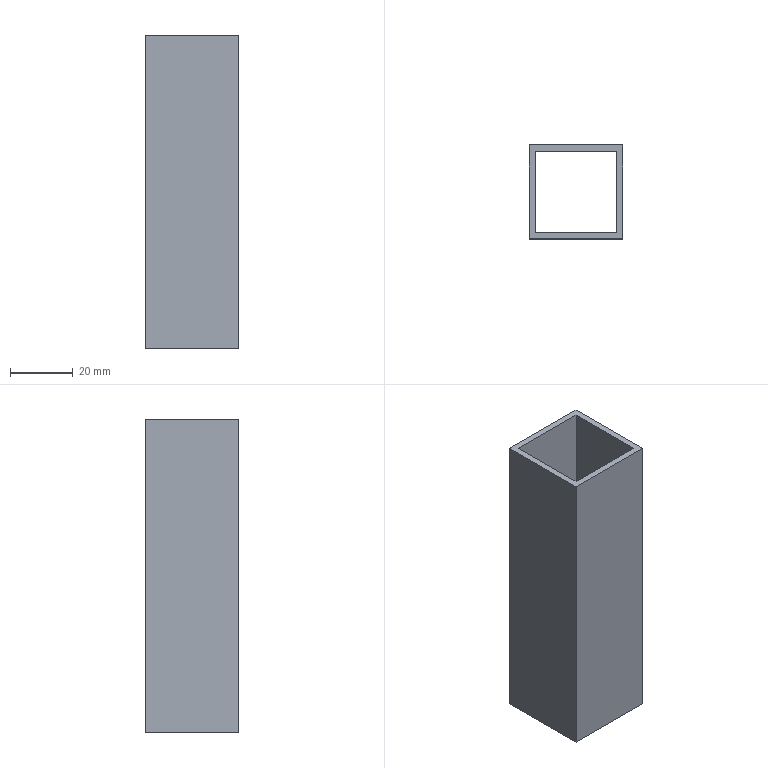Part | SolidWorks | features Extrusion 1 | 1 solid | 10 faces | box 30 x 30 x 100 mm | volume 22400 mm3 | plane 10
STEP:
#1=CARTESIAN_POINT('',(-15.,15.,50.));
#2=VERTEX_POINT('',#1);
#3=CARTESIAN_POINT('',(-15.,-15.,50.));
#4=VERTEX_POINT('',#3);
#5=CARTESIAN_POINT('',(-15.,-15.,50.));
#6=DIRECTION('',(0.,-1.,0.));
#7=VECTOR('',#6,1000.);
#8=LINE('',#5,#7);
#9=EDGE_CURVE('',#2,#4,#8,.T.);
#10=ORIENTED_EDGE('',*,*,#9,.T.);
#11=CARTESIAN_POINT('',(15.,-15.,50.));
#12=VERTEX_POINT('',#11);
#13=CARTESIAN_POINT('',(15.,-15.,50.));
#14=DIRECTION('',(1.,0.,0.));
#15=VECTOR('',#14,1000.);
#16=LINE('',#13,#15);
#17=EDGE_CURVE('',#4,#12,#16,.T.);
#18=ORIENTED_EDGE('',*,*,#17,.T.);
#19=CARTESIAN_POINT('',(15.,15.,50.));
#20=VERTEX_POINT('',#19);
#21=CARTESIAN_POINT('',(15.,-15.,50.));
#22=DIRECTION('',(0.,1.,0.));
#23=VECTOR('',#22,1000.);
#24=LINE('',#21,#23);
#25=EDGE_CURVE('',#12,#20,#24,.T.);
#26=ORIENTED_EDGE('',*,*,#25,.T.);
#27=CARTESIAN_POINT('',(15.,15.,50.));
#28=DIRECTION('',(-1.,0.,0.));
#29=VECTOR('',#28,1000.);
#30=LINE('',#27,#29);
#31=EDGE_CURVE('',#20,#2,#30,.T.);
#32=ORIENTED_EDGE('',*,*,#31,.T.);
#33=EDGE_LOOP('',(#10,#18,#26,#32));
#34=FACE_OUTER_BOUND('',#33,.T.);
#35=CARTESIAN_POINT('',(13.,-13.,50.));
#36=VERTEX_POINT('',#35);
#37=CARTESIAN_POINT('',(13.,13.,50.));
#38=VERTEX_POINT('',#37);
#39=CARTESIAN_POINT('',(13.,-13.,50.));
#40=DIRECTION('',(0.,1.,0.));
#41=VECTOR('',#40,1000.);
#42=LINE('',#39,#41);
#43=EDGE_CURVE('',#36,#38,#42,.T.);
#44=ORIENTED_EDGE('',*,*,#43,.F.);
#45=CARTESIAN_POINT('',(-13.,-13.,50.));
#46=VERTEX_POINT('',#45);
#47=CARTESIAN_POINT('',(13.,-13.,50.));
#48=DIRECTION('',(1.,0.,0.));
#49=VECTOR('',#48,1000.);
#50=LINE('',#47,#49);
#51=EDGE_CURVE('',#46,#36,#50,.T.);
#52=ORIENTED_EDGE('',*,*,#51,.F.);
#53=CARTESIAN_POINT('',(-13.,13.,50.));
#54=VERTEX_POINT('',#53);
#55=CARTESIAN_POINT('',(-13.,-13.,50.));
#56=DIRECTION('',(0.,-1.,0.));
#57=VECTOR('',#56,1000.);
#58=LINE('',#55,#57);
#59=EDGE_CURVE('',#54,#46,#58,.T.);
#60=ORIENTED_EDGE('',*,*,#59,.F.);
#61=CARTESIAN_POINT('',(13.,13.,50.));
#62=DIRECTION('',(-1.,0.,0.));
#63=VECTOR('',#62,1000.);
#64=LINE('',#61,#63);
#65=EDGE_CURVE('',#38,#54,#64,.T.);
#66=ORIENTED_EDGE('',*,*,#65,.F.);
#67=EDGE_LOOP('',(#44,#52,#60,#66));
#68=FACE_BOUND('',#67,.T.);
#69=CARTESIAN_POINT('',(0.,0.,50.));
#70=DIRECTION('',(0.,0.,1.));
#71=DIRECTION('',(1.,0.,0.));
#72=AXIS2_PLACEMENT_3D('',#69,#70,#71);
#73=PLANE('',#72);
#74=ADVANCED_FACE('',(#34,#68),#73,.T.);
#75=CARTESIAN_POINT('',(-15.,15.,-50.));
#76=VERTEX_POINT('',#75);
#77=CARTESIAN_POINT('',(-15.,-15.,-50.));
#78=VERTEX_POINT('',#77);
#79=CARTESIAN_POINT('',(-15.,-15.,-50.));
#80=DIRECTION('',(0.,-1.,0.));
#81=VECTOR('',#80,1000.);
#82=LINE('',#79,#81);
#83=EDGE_CURVE('',#76,#78,#82,.T.);
#84=ORIENTED_EDGE('',*,*,#83,.F.);
#85=CARTESIAN_POINT('',(15.,15.,-50.));
#86=VERTEX_POINT('',#85);
#87=CARTESIAN_POINT('',(15.,15.,-50.));
#88=DIRECTION('',(-1.,0.,0.));
#89=VECTOR('',#88,1000.);
#90=LINE('',#87,#89);
#91=EDGE_CURVE('',#86,#76,#90,.T.);
#92=ORIENTED_EDGE('',*,*,#91,.F.);
#93=CARTESIAN_POINT('',(15.,-15.,-50.));
#94=VERTEX_POINT('',#93);
#95=CARTESIAN_POINT('',(15.,-15.,-50.));
#96=DIRECTION('',(0.,1.,0.));
#97=VECTOR('',#96,1000.);
#98=LINE('',#95,#97);
#99=EDGE_CURVE('',#94,#86,#98,.T.);
#100=ORIENTED_EDGE('',*,*,#99,.F.);
#101=CARTESIAN_POINT('',(15.,-15.,-50.));
#102=DIRECTION('',(1.,0.,0.));
#103=VECTOR('',#102,1000.);
#104=LINE('',#101,#103);
#105=EDGE_CURVE('',#78,#94,#104,.T.);
#106=ORIENTED_EDGE('',*,*,#105,.F.);
#107=EDGE_LOOP('',(#84,#92,#100,#106));
#108=FACE_OUTER_BOUND('',#107,.T.);
#109=CARTESIAN_POINT('',(-13.,-13.,-50.));
#110=VERTEX_POINT('',#109);
#111=CARTESIAN_POINT('',(13.,-13.,-50.));
#112=VERTEX_POINT('',#111);
#113=CARTESIAN_POINT('',(13.,-13.,-50.));
#114=DIRECTION('',(1.,0.,0.));
#115=VECTOR('',#114,1000.);
#116=LINE('',#113,#115);
#117=EDGE_CURVE('',#110,#112,#116,.T.);
#118=ORIENTED_EDGE('',*,*,#117,.T.);
#119=CARTESIAN_POINT('',(13.,13.,-50.));
#120=VERTEX_POINT('',#119);
#121=CARTESIAN_POINT('',(13.,-13.,-50.));
#122=DIRECTION('',(0.,1.,0.));
#123=VECTOR('',#122,1000.);
#124=LINE('',#121,#123);
#125=EDGE_CURVE('',#112,#120,#124,.T.);
#126=ORIENTED_EDGE('',*,*,#125,.T.);
#127=CARTESIAN_POINT('',(-13.,13.,-50.));
#128=VERTEX_POINT('',#127);
#129=CARTESIAN_POINT('',(13.,13.,-50.));
#130=DIRECTION('',(-1.,0.,0.));
#131=VECTOR('',#130,1000.);
#132=LINE('',#129,#131);
#133=EDGE_CURVE('',#120,#128,#132,.T.);
#134=ORIENTED_EDGE('',*,*,#133,.T.);
#135=CARTESIAN_POINT('',(-13.,-13.,-50.));
#136=DIRECTION('',(0.,-1.,0.));
#137=VECTOR('',#136,1000.);
#138=LINE('',#135,#137);
#139=EDGE_CURVE('',#128,#110,#138,.T.);
#140=ORIENTED_EDGE('',*,*,#139,.T.);
#141=EDGE_LOOP('',(#118,#126,#134,#140));
#142=FACE_BOUND('',#141,.T.);
#143=CARTESIAN_POINT('',(0.,0.,-50.));
#144=DIRECTION('',(0.,0.,1.));
#145=DIRECTION('',(1.,0.,0.));
#146=AXIS2_PLACEMENT_3D('',#143,#144,#145);
#147=PLANE('',#146);
#148=ADVANCED_FACE('',(#108,#142),#147,.F.);
#149=ORIENTED_EDGE('',*,*,#83,.T.);
#150=CARTESIAN_POINT('',(-15.,-15.,50.));
#151=DIRECTION('',(0.,0.,-1.));
#152=VECTOR('',#151,1000.);
#153=LINE('',#150,#152);
#154=EDGE_CURVE('',#4,#78,#153,.T.);
#155=ORIENTED_EDGE('',*,*,#154,.F.);
#156=ORIENTED_EDGE('',*,*,#9,.F.);
#157=CARTESIAN_POINT('',(-15.,15.,50.));
#158=DIRECTION('',(0.,0.,-1.));
#159=VECTOR('',#158,1000.);
#160=LINE('',#157,#159);
#161=EDGE_CURVE('',#2,#76,#160,.T.);
#162=ORIENTED_EDGE('',*,*,#161,.T.);
#163=EDGE_LOOP('',(#149,#155,#156,#162));
#164=FACE_OUTER_BOUND('',#163,.T.);
#165=CARTESIAN_POINT('',(-15.,-15.,50.));
#166=DIRECTION('',(1.,0.,0.));
#167=DIRECTION('',(0.,1.,0.));
#168=AXIS2_PLACEMENT_3D('',#165,#166,#167);
#169=PLANE('',#168);
#170=ADVANCED_FACE('',(#164),#169,.F.);
#171=ORIENTED_EDGE('',*,*,#105,.T.);
#172=CARTESIAN_POINT('',(15.,-15.,50.));
#173=DIRECTION('',(0.,0.,-1.));
#174=VECTOR('',#173,1000.);
#175=LINE('',#172,#174);
#176=EDGE_CURVE('',#12,#94,#175,.T.);
#177=ORIENTED_EDGE('',*,*,#176,.F.);
#178=ORIENTED_EDGE('',*,*,#17,.F.);
#179=ORIENTED_EDGE('',*,*,#154,.T.);
#180=EDGE_LOOP('',(#171,#177,#178,#179));
#181=FACE_OUTER_BOUND('',#180,.T.);
#182=CARTESIAN_POINT('',(15.,-15.,50.));
#183=DIRECTION('',(0.,1.,0.));
#184=DIRECTION('',(-1.,0.,0.));
#185=AXIS2_PLACEMENT_3D('',#182,#183,#184);
#186=PLANE('',#185);
#187=ADVANCED_FACE('',(#181),#186,.F.);
#188=ORIENTED_EDGE('',*,*,#99,.T.);
#189=CARTESIAN_POINT('',(15.,15.,50.));
#190=DIRECTION('',(0.,0.,-1.));
#191=VECTOR('',#190,1000.);
#192=LINE('',#189,#191);
#193=EDGE_CURVE('',#20,#86,#192,.T.);
#194=ORIENTED_EDGE('',*,*,#193,.F.);
#195=ORIENTED_EDGE('',*,*,#25,.F.);
#196=ORIENTED_EDGE('',*,*,#176,.T.);
#197=EDGE_LOOP('',(#188,#194,#195,#196));
#198=FACE_OUTER_BOUND('',#197,.T.);
#199=CARTESIAN_POINT('',(15.,-15.,50.));
#200=DIRECTION('',(-1.,0.,0.));
#201=DIRECTION('',(0.,0.,1.));
#202=AXIS2_PLACEMENT_3D('',#199,#200,#201);
#203=PLANE('',#202);
#204=ADVANCED_FACE('',(#198),#203,.F.);
#205=ORIENTED_EDGE('',*,*,#91,.T.);
#206=ORIENTED_EDGE('',*,*,#161,.F.);
#207=ORIENTED_EDGE('',*,*,#31,.F.);
#208=ORIENTED_EDGE('',*,*,#193,.T.);
#209=EDGE_LOOP('',(#205,#206,#207,#208));
#210=FACE_OUTER_BOUND('',#209,.T.);
#211=CARTESIAN_POINT('',(15.,15.,50.));
#212=DIRECTION('',(0.,-1.,0.));
#213=DIRECTION('',(0.,0.,-1.));
#214=AXIS2_PLACEMENT_3D('',#211,#212,#213);
#215=PLANE('',#214);
#216=ADVANCED_FACE('',(#210),#215,.F.);
#217=ORIENTED_EDGE('',*,*,#117,.F.);
#218=CARTESIAN_POINT('',(-13.,-13.,50.));
#219=DIRECTION('',(0.,0.,-1.));
#220=VECTOR('',#219,1000.);
#221=LINE('',#218,#220);
#222=EDGE_CURVE('',#46,#110,#221,.T.);
#223=ORIENTED_EDGE('',*,*,#222,.F.);
#224=ORIENTED_EDGE('',*,*,#51,.T.);
#225=CARTESIAN_POINT('',(13.,-13.,50.));
#226=DIRECTION('',(0.,0.,-1.));
#227=VECTOR('',#226,1000.);
#228=LINE('',#225,#227);
#229=EDGE_CURVE('',#36,#112,#228,.T.);
#230=ORIENTED_EDGE('',*,*,#229,.T.);
#231=EDGE_LOOP('',(#217,#223,#224,#230));
#232=FACE_OUTER_BOUND('',#231,.T.);
#233=CARTESIAN_POINT('',(13.,-13.,50.));
#234=DIRECTION('',(0.,1.,0.));
#235=DIRECTION('',(0.,0.,1.));
#236=AXIS2_PLACEMENT_3D('',#233,#234,#235);
#237=PLANE('',#236);
#238=ADVANCED_FACE('',(#232),#237,.T.);
#239=ORIENTED_EDGE('',*,*,#125,.F.);
#240=ORIENTED_EDGE('',*,*,#229,.F.);
#241=ORIENTED_EDGE('',*,*,#43,.T.);
#242=CARTESIAN_POINT('',(13.,13.,50.));
#243=DIRECTION('',(0.,0.,-1.));
#244=VECTOR('',#243,1000.);
#245=LINE('',#242,#244);
#246=EDGE_CURVE('',#38,#120,#245,.T.);
#247=ORIENTED_EDGE('',*,*,#246,.T.);
#248=EDGE_LOOP('',(#239,#240,#241,#247));
#249=FACE_OUTER_BOUND('',#248,.T.);
#250=CARTESIAN_POINT('',(13.,-13.,50.));
#251=DIRECTION('',(-1.,0.,0.));
#252=DIRECTION('',(0.,0.,1.));
#253=AXIS2_PLACEMENT_3D('',#250,#251,#252);
#254=PLANE('',#253);
#255=ADVANCED_FACE('',(#249),#254,.T.);
#256=ORIENTED_EDGE('',*,*,#133,.F.);
#257=ORIENTED_EDGE('',*,*,#246,.F.);
#258=ORIENTED_EDGE('',*,*,#65,.T.);
#259=CARTESIAN_POINT('',(-13.,13.,50.));
#260=DIRECTION('',(0.,0.,-1.));
#261=VECTOR('',#260,1000.);
#262=LINE('',#259,#261);
#263=EDGE_CURVE('',#54,#128,#262,.T.);
#264=ORIENTED_EDGE('',*,*,#263,.T.);
#265=EDGE_LOOP('',(#256,#257,#258,#264));
#266=FACE_OUTER_BOUND('',#265,.T.);
#267=CARTESIAN_POINT('',(13.,13.,50.));
#268=DIRECTION('',(0.,-1.,0.));
#269=DIRECTION('',(0.,0.,-1.));
#270=AXIS2_PLACEMENT_3D('',#267,#268,#269);
#271=PLANE('',#270);
#272=ADVANCED_FACE('',(#266),#271,.T.);
#273=ORIENTED_EDGE('',*,*,#139,.F.);
#274=ORIENTED_EDGE('',*,*,#263,.F.);
#275=ORIENTED_EDGE('',*,*,#59,.T.);
#276=ORIENTED_EDGE('',*,*,#222,.T.);
#277=EDGE_LOOP('',(#273,#274,#275,#276));
#278=FACE_OUTER_BOUND('',#277,.T.);
#279=CARTESIAN_POINT('',(-13.,-13.,50.));
#280=DIRECTION('',(1.,0.,0.));
#281=DIRECTION('',(0.,0.,-1.));
#282=AXIS2_PLACEMENT_3D('',#279,#280,#281);
#283=PLANE('',#282);
#284=ADVANCED_FACE('',(#278),#283,.T.);
#285=CLOSED_SHELL('',(#74,#148,#170,#187,#204,#216,#238,#255,#272,#284));
#286=MANIFOLD_SOLID_BREP('',#285);
#287=CARTESIAN_POINT('',(0.,0.,0.));
#288=DIRECTION('',(0.,0.,1.));
#289=DIRECTION('',(1.,0.,0.));
#290=AXIS2_PLACEMENT_3D('',#287,#288,#289);
#291=(LENGTH_UNIT()NAMED_UNIT(*)SI_UNIT(.MILLI.,.METRE.));
#292=UNCERTAINTY_MEASURE_WITH_UNIT(LENGTH_MEASURE(0.00001),#291,'','');
#293=(NAMED_UNIT(*)PLANE_ANGLE_UNIT()SI_UNIT($,.RADIAN.));
#294=(NAMED_UNIT(*)SI_UNIT($,.STERADIAN.)SOLID_ANGLE_UNIT());
#295=(GEOMETRIC_REPRESENTATION_CONTEXT(3)GLOBAL_UNCERTAINTY_ASSIGNED_CONTEXT((#292))GLOBAL_UNIT_ASSIGNED_CONTEXT((#291,#293,#294))REPRESENTATION_CONTEXT('',''));
#296=ADVANCED_BREP_SHAPE_REPRESENTATION('',(#286,#290),#295);